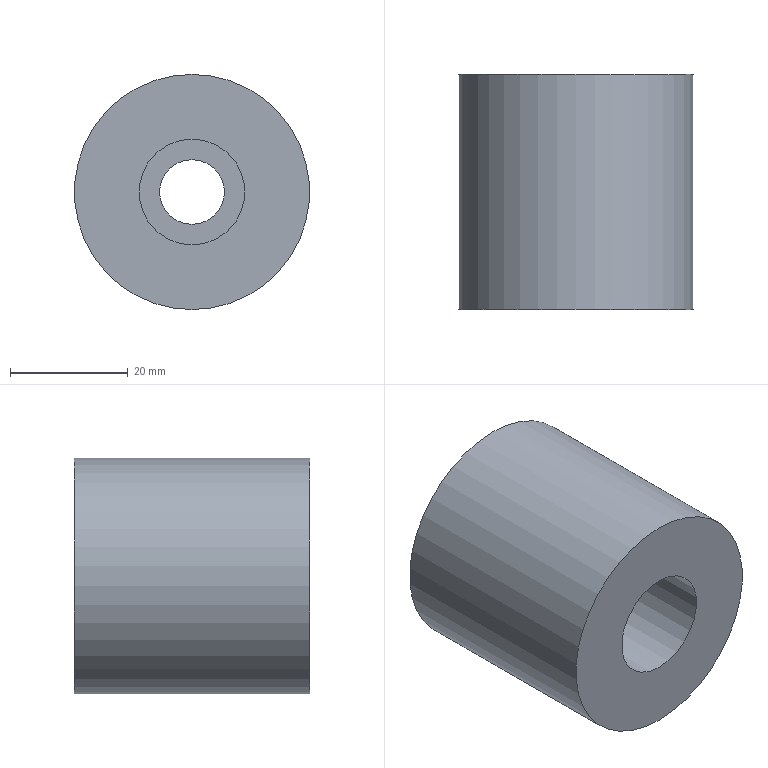Part | NX | features solid 2 | 1 solid | 6 faces | box 40 x 40 x 40 mm | volume 41681 mm3 | cylinder 3 | plane 3 | commonest cylinder face diameters 11 x1 18 x1 40 x1
STEP:
#1=CARTESIAN_POINT('',(0.,140.,-210.));
#2=VERTEX_POINT('',#1);
#3=CARTESIAN_POINT('',(0.,140.,-190.));
#4=DIRECTION('',(0.,-1.,0.));
#5=DIRECTION('',(0.,0.,-1.));
#6=AXIS2_PLACEMENT_3D('',#3,#4,#5);
#7=CIRCLE('',#6,20.);
#8=EDGE_CURVE('',#2,#2,#7,.T.);
#9=ORIENTED_EDGE('',*,*,#8,.T.);
#10=EDGE_LOOP('',(#9));
#11=FACE_BOUND('',#10,.T.);
#12=CARTESIAN_POINT('',(0.,100.,-210.));
#13=VERTEX_POINT('',#12);
#14=CARTESIAN_POINT('',(0.,100.,-190.));
#15=DIRECTION('',(0.,-1.,0.));
#16=DIRECTION('',(0.,0.,-1.));
#17=AXIS2_PLACEMENT_3D('',#14,#15,#16);
#18=CIRCLE('',#17,20.);
#19=EDGE_CURVE('',#13,#13,#18,.T.);
#20=ORIENTED_EDGE('',*,*,#19,.F.);
#21=EDGE_LOOP('',(#20));
#22=FACE_BOUND('',#21,.T.);
#23=CARTESIAN_POINT('',(0.,140.,-190.));
#24=DIRECTION('',(0.,-1.,0.));
#25=DIRECTION('',(0.,0.,-1.));
#26=AXIS2_PLACEMENT_3D('',#23,#24,#25);
#27=CYLINDRICAL_SURFACE('',#26,20.);
#28=ADVANCED_FACE('',(#11,#22),#27,.T.);
#29=CARTESIAN_POINT('',(0.,140.,-195.5));
#30=VERTEX_POINT('',#29);
#31=CARTESIAN_POINT('',(0.,140.,-190.));
#32=DIRECTION('',(0.,-1.,0.));
#33=DIRECTION('',(0.,0.,-1.));
#34=AXIS2_PLACEMENT_3D('',#31,#32,#33);
#35=CIRCLE('',#34,5.5);
#36=EDGE_CURVE('',#30,#30,#35,.T.);
#37=ORIENTED_EDGE('',*,*,#36,.T.);
#38=EDGE_LOOP('',(#37));
#39=FACE_BOUND('',#38,.T.);
#40=ORIENTED_EDGE('',*,*,#8,.F.);
#41=EDGE_LOOP('',(#40));
#42=FACE_BOUND('',#41,.T.);
#43=CARTESIAN_POINT('',(0.,140.,-190.));
#44=DIRECTION('',(0.,-1.,0.));
#45=DIRECTION('',(0.,0.,-1.));
#46=AXIS2_PLACEMENT_3D('',#43,#44,#45);
#47=PLANE('',#46);
#48=ADVANCED_FACE('',(#39,#42),#47,.F.);
#49=CARTESIAN_POINT('',(0.,100.,-181.));
#50=VERTEX_POINT('',#49);
#51=CARTESIAN_POINT('',(0.,100.,-190.));
#52=DIRECTION('',(0.,1.,0.));
#53=DIRECTION('',(0.,0.,1.));
#54=AXIS2_PLACEMENT_3D('',#51,#52,#53);
#55=CIRCLE('',#54,9.);
#56=EDGE_CURVE('',#50,#50,#55,.T.);
#57=ORIENTED_EDGE('',*,*,#56,.T.);
#58=EDGE_LOOP('',(#57));
#59=FACE_BOUND('',#58,.T.);
#60=ORIENTED_EDGE('',*,*,#19,.T.);
#61=EDGE_LOOP('',(#60));
#62=FACE_BOUND('',#61,.T.);
#63=CARTESIAN_POINT('',(0.,100.,-190.));
#64=DIRECTION('',(0.,-1.,0.));
#65=DIRECTION('',(0.,0.,-1.));
#66=AXIS2_PLACEMENT_3D('',#63,#64,#65);
#67=PLANE('',#66);
#68=ADVANCED_FACE('',(#59,#62),#67,.T.);
#69=CARTESIAN_POINT('',(0.,130.,-184.5));
#70=VERTEX_POINT('',#69);
#71=CARTESIAN_POINT('',(0.,130.,-190.));
#72=DIRECTION('',(0.,1.,0.));
#73=DIRECTION('',(0.,0.,1.));
#74=AXIS2_PLACEMENT_3D('',#71,#72,#73);
#75=CIRCLE('',#74,5.5);
#76=EDGE_CURVE('',#70,#70,#75,.T.);
#77=ORIENTED_EDGE('',*,*,#76,.F.);
#78=EDGE_LOOP('',(#77));
#79=FACE_BOUND('',#78,.T.);
#80=ORIENTED_EDGE('',*,*,#36,.F.);
#81=EDGE_LOOP('',(#80));
#82=FACE_BOUND('',#81,.T.);
#83=CARTESIAN_POINT('',(0.,150.,-190.));
#84=DIRECTION('',(0.,1.,0.));
#85=DIRECTION('',(0.,0.,1.));
#86=AXIS2_PLACEMENT_3D('',#83,#84,#85);
#87=CYLINDRICAL_SURFACE('',#86,5.5);
#88=ADVANCED_FACE('',(#79,#82),#87,.F.);
#89=ORIENTED_EDGE('',*,*,#76,.T.);
#90=EDGE_LOOP('',(#89));
#91=FACE_BOUND('',#90,.T.);
#92=CARTESIAN_POINT('',(0.,130.,-181.));
#93=VERTEX_POINT('',#92);
#94=CARTESIAN_POINT('',(0.,130.,-190.));
#95=DIRECTION('',(0.,1.,0.));
#96=DIRECTION('',(0.,0.,1.));
#97=AXIS2_PLACEMENT_3D('',#94,#95,#96);
#98=CIRCLE('',#97,9.);
#99=EDGE_CURVE('',#93,#93,#98,.T.);
#100=ORIENTED_EDGE('',*,*,#99,.F.);
#101=EDGE_LOOP('',(#100));
#102=FACE_BOUND('',#101,.T.);
#103=CARTESIAN_POINT('',(0.,130.,-190.));
#104=DIRECTION('',(0.,1.,0.));
#105=DIRECTION('',(0.,0.,1.));
#106=AXIS2_PLACEMENT_3D('',#103,#104,#105);
#107=PLANE('',#106);
#108=ADVANCED_FACE('',(#91,#102),#107,.F.);
#109=ORIENTED_EDGE('',*,*,#99,.T.);
#110=EDGE_LOOP('',(#109));
#111=FACE_BOUND('',#110,.T.);
#112=ORIENTED_EDGE('',*,*,#56,.F.);
#113=EDGE_LOOP('',(#112));
#114=FACE_BOUND('',#113,.T.);
#115=CARTESIAN_POINT('',(0.,100.,-190.));
#116=DIRECTION('',(0.,1.,0.));
#117=DIRECTION('',(0.,0.,1.));
#118=AXIS2_PLACEMENT_3D('',#115,#116,#117);
#119=CYLINDRICAL_SURFACE('',#118,9.);
#120=ADVANCED_FACE('',(#111,#114),#119,.F.);
#121=CLOSED_SHELL('',(#28,#48,#68,#88,#108,#120));
#122=MANIFOLD_SOLID_BREP('',#121);
#123=(LENGTH_UNIT()NAMED_UNIT(*)SI_UNIT(.MILLI.,.METRE.));
#124=UNCERTAINTY_MEASURE_WITH_UNIT(LENGTH_MEASURE(0.00001),#123,'','');
#125=(NAMED_UNIT(*)PLANE_ANGLE_UNIT()SI_UNIT($,.RADIAN.));
#126=(NAMED_UNIT(*)SI_UNIT($,.STERADIAN.)SOLID_ANGLE_UNIT());
#127=(GEOMETRIC_REPRESENTATION_CONTEXT(3)GLOBAL_UNCERTAINTY_ASSIGNED_CONTEXT((#124))GLOBAL_UNIT_ASSIGNED_CONTEXT((#123,#125,#126))REPRESENTATION_CONTEXT('',''));
#128=ADVANCED_BREP_SHAPE_REPRESENTATION('',(#122),#127);